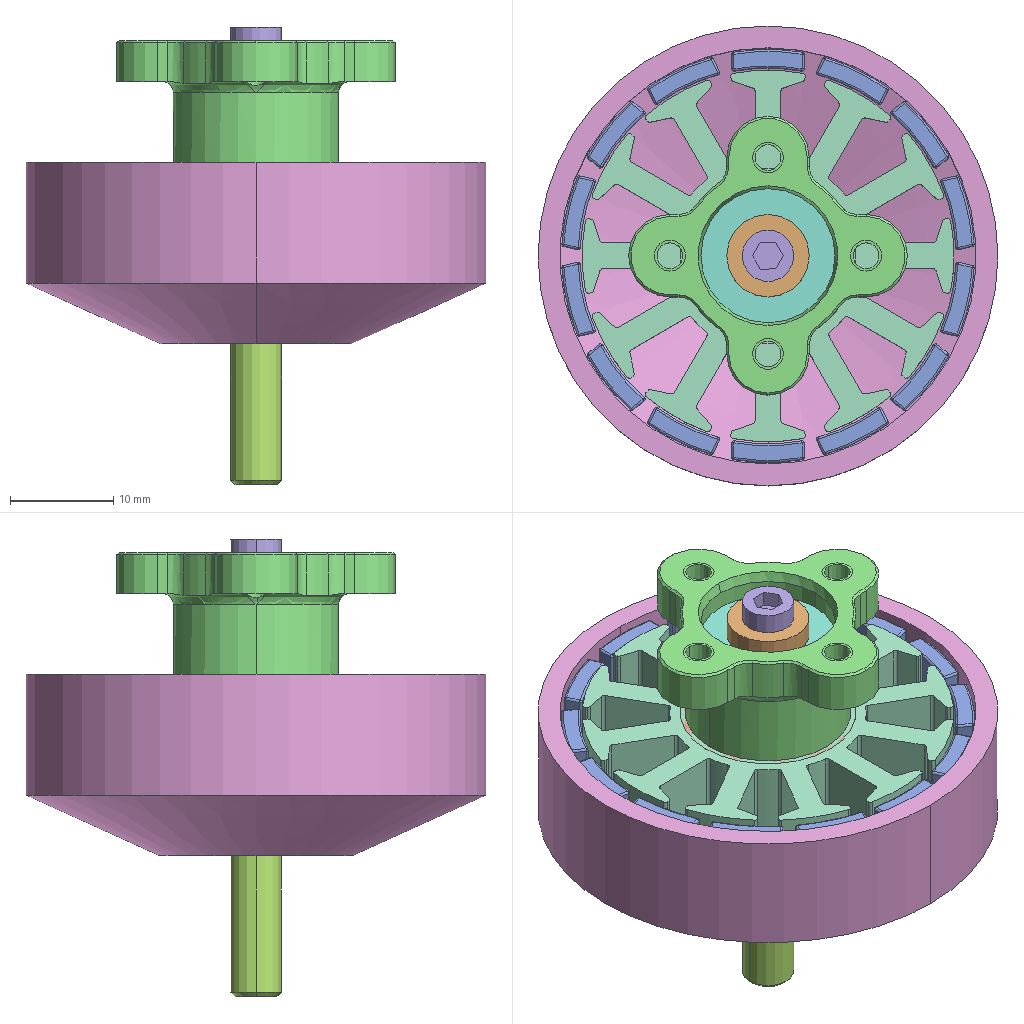Assembly | SolidWorks | 8 different items | 21 placed | box 45 x 45 x 44 mm
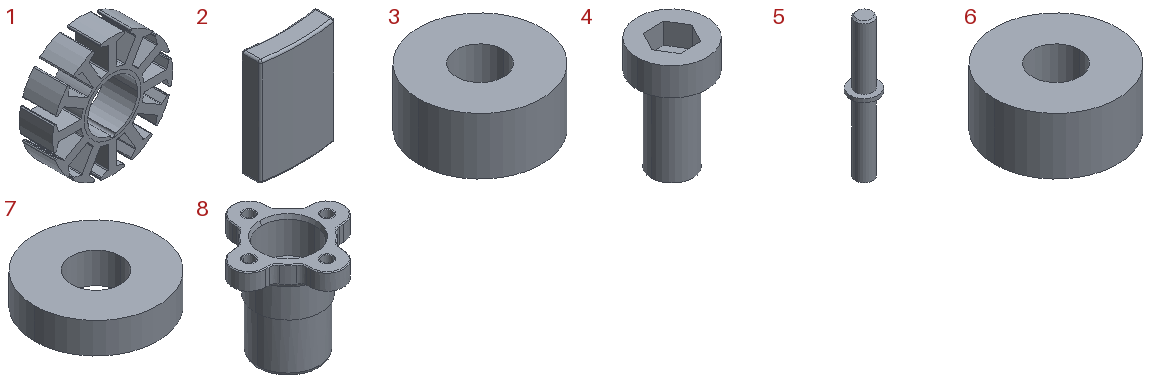Parts list (item | quantity | size | volume | features):
1 | x1 | - | - | features BaseBody 1, RefSurface 1
2 | x14 | 7 x 2.098 x 10 mm | 126.049 mm3 | features BaseBody 1
3 | x1 | 13 x 13 x 6 mm | 678.584 mm3 | features Extrusion 1
4 | x1 | 5 x 5 x 8 mm | 72.989 mm3 | features Cut 1, Extrusion 1, ICE 1
5 | x1 | 8 x 8 x 40 mm | 765.722 mm3 | features ICE 2, 3DProfileFeature 1, Extrusion 1, HoleWzd 1, StudWizard 1
6 | x1 | 13 x 13 x 6 mm | 678.584 mm3 | features Extrusion 1
7 | x1 | 8 x 8 x 2 mm | 84.446 mm3 | features Extrusion 1
8 | x1 | - | - | features RefSurface 4, BaseBody 1
Mates (type | each side: item.copy, entity, surface, feature):
Concentric | 8.1 edge | 1.1 edge
Coincident | 8.1 face plane Input 1 | 1.1 edge
InPlace | 8.1 face plane Input 1 | 6.1 plane
Concentric | 1.1 edge | 2.1 edge
InPlace | 6.1 face plane Boss-Extrude1 | 5.1 plane
InPlace | 8.1 face plane Input 1 | 3.1 plane
InPlace | 3.1 face plane Boss-Extrude1 | 7.1 plane
InPlace | 7.1 face plane Boss-Extrude1 | 4.1 plane